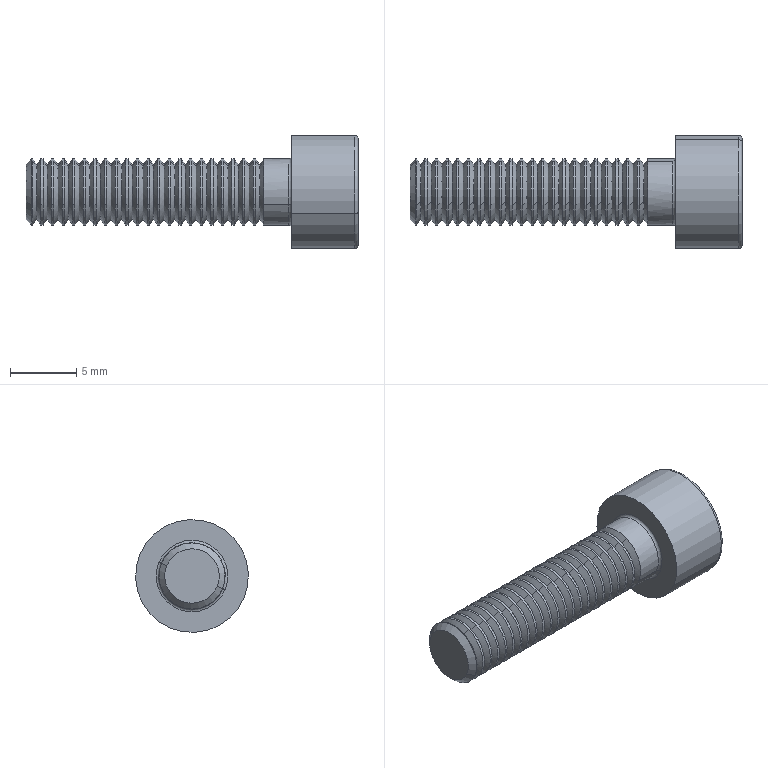Part | STEP file | Socket Head Cap Screw_ISO(ISO 4762 M5 x 20 --- 20S)_Valor predeterminado | 1 solid | 159 faces | box 25 x 8.5 x 8.5 mm | volume 588.412 mm3 | cone 92 | cylinder 48 | plane 15 | torus 4 | commonest cylinder face diameters 5 x46 8.5 x2